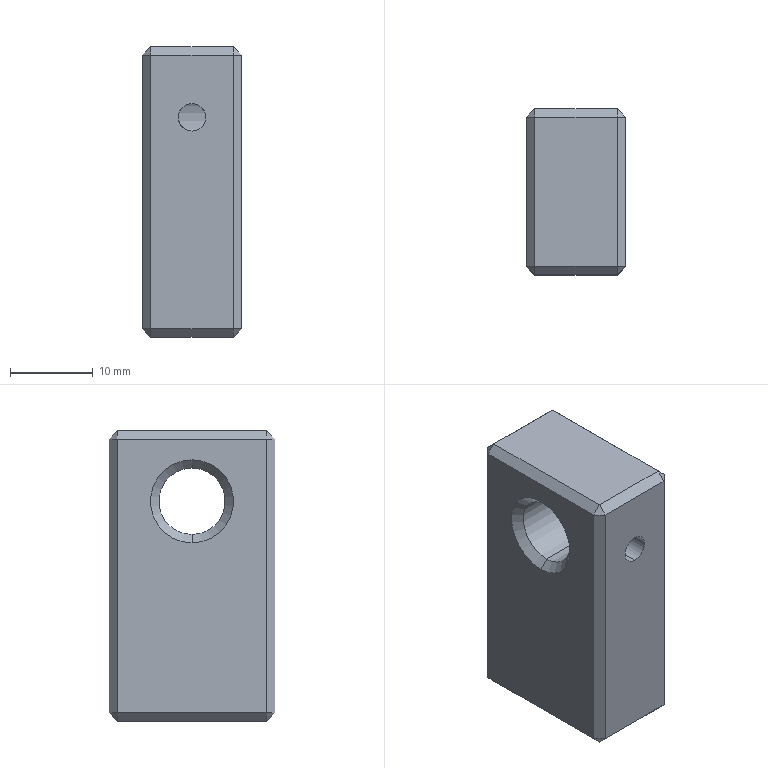Part | STEP file | BPSP-11-14 Pusher Shaft Fixing Plate_Default | 1 solid | 42 faces | box 12 x 20 x 35 mm | volume 7342 mm3 | plane 26 | cylinder 8 | cone 8 | commonest cylinder face diameters 3.3 x6 8 x2